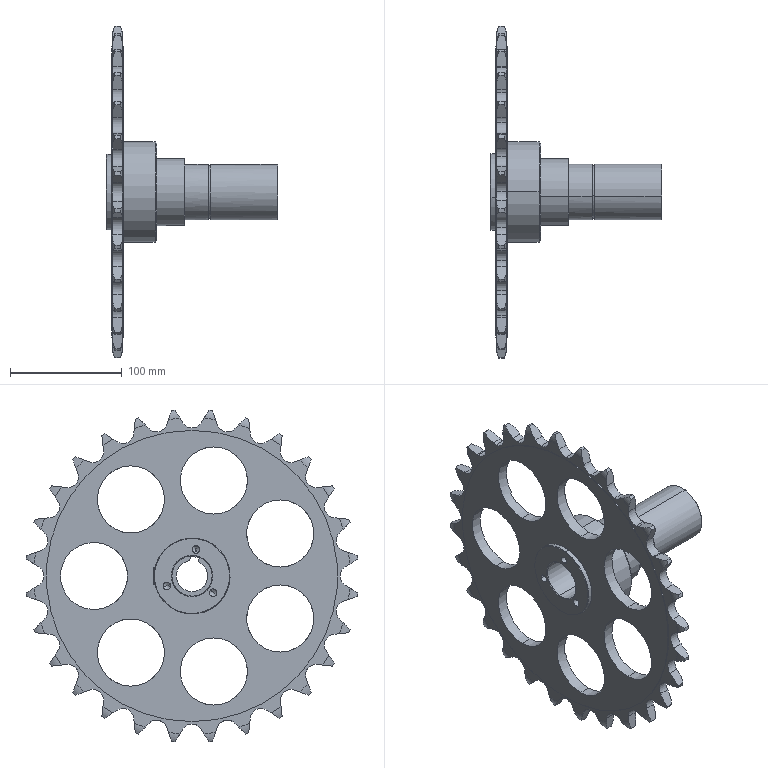Part | STEP file | 101000007733 | 2 solids | 312 faces | box 153 x 296.456 x 296.456 mm | volume 689449 mm3 | cylinder 135 | plane 87 | torus 56 | cone 26 | spline 8 | commonest cylinder face diameters 19.05 x46 298 x28 60 x19 6.8 x8 165 x7 185 x7